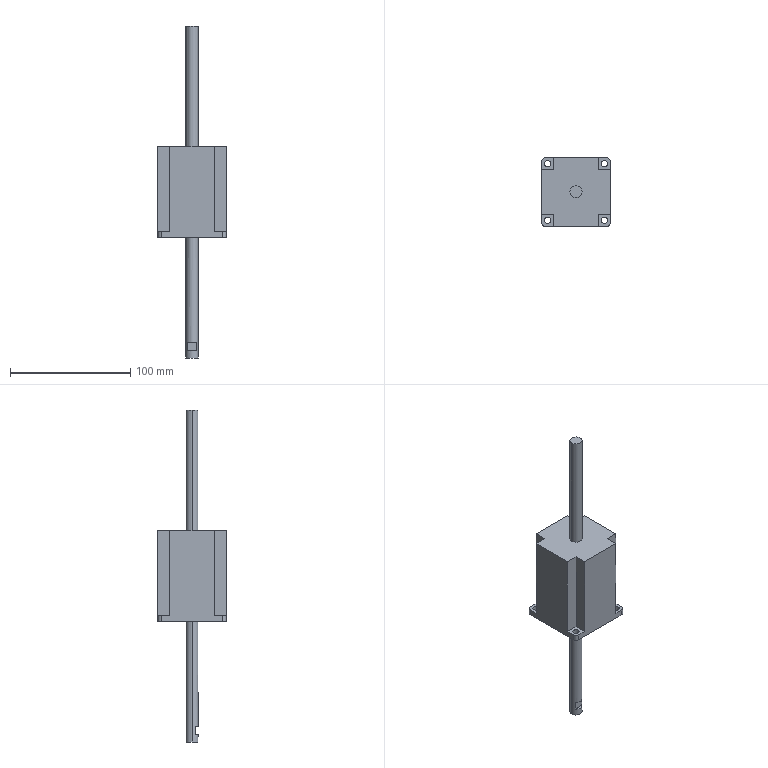Part | SolidWorks | features ICE 6, Extrusion 1, Fillet 1, MoveFace 1 | 1 solid | 39 faces | box 57 x 57 x 276 mm | volume 233690 mm3 | plane 23 | cylinder 16 | commonest cylinder face diameters 5.2 x8 6 x4 10 x4
STEP:
#1=CARTESIAN_POINT('',(5.,0.,176.));
#2=VERTEX_POINT('',#1);
#3=CARTESIAN_POINT('',(-5.,0.,176.));
#4=VERTEX_POINT('',#3);
#5=CARTESIAN_POINT('',(0.,0.,176.));
#6=DIRECTION('',(0.,0.,1.));
#7=DIRECTION('',(1.,0.,0.));
#8=AXIS2_PLACEMENT_3D('',#5,#6,#7);
#9=CIRCLE('',#8,5.);
#10=EDGE_CURVE('',#2,#4,#9,.T.);
#11=ORIENTED_EDGE('',*,*,#10,.F.);
#12=CARTESIAN_POINT('',(5.,0.,76.));
#13=VERTEX_POINT('',#12);
#14=CARTESIAN_POINT('',(5.,0.,256.));
#15=DIRECTION('',(0.,0.,-1.));
#16=VECTOR('',#15,1000.);
#17=LINE('',#14,#16);
#18=EDGE_CURVE('',#2,#13,#17,.T.);
#19=ORIENTED_EDGE('',*,*,#18,.T.);
#20=CARTESIAN_POINT('',(-5.,0.,76.));
#21=VERTEX_POINT('',#20);
#22=CARTESIAN_POINT('',(0.,0.,76.));
#23=DIRECTION('',(0.,0.,1.));
#24=DIRECTION('',(-1.,0.,0.));
#25=AXIS2_PLACEMENT_3D('',#22,#23,#24);
#26=CIRCLE('',#25,5.);
#27=EDGE_CURVE('',#13,#21,#26,.T.);
#28=ORIENTED_EDGE('',*,*,#27,.T.);
#29=CARTESIAN_POINT('',(-5.,0.,256.));
#30=DIRECTION('',(0.,0.,-1.));
#31=VECTOR('',#30,1000.);
#32=LINE('',#29,#31);
#33=EDGE_CURVE('',#4,#21,#32,.T.);
#34=ORIENTED_EDGE('',*,*,#33,.F.);
#35=EDGE_LOOP('',(#11,#19,#28,#34));
#36=FACE_OUTER_BOUND('',#35,.T.);
#37=CARTESIAN_POINT('',(0.,0.,256.));
#38=DIRECTION('',(0.,0.,-1.));
#39=DIRECTION('',(-1.,0.,0.));
#40=AXIS2_PLACEMENT_3D('',#37,#38,#39);
#41=CYLINDRICAL_SURFACE('',#40,5.);
#42=ADVANCED_FACE('',(#36),#41,.T.);
#43=CARTESIAN_POINT('',(26.15,-23.55,5.));
#44=VERTEX_POINT('',#43);
#45=CARTESIAN_POINT('',(20.95,-23.55,5.));
#46=VERTEX_POINT('',#45);
#47=CARTESIAN_POINT('',(23.55,-23.55,5.));
#48=DIRECTION('',(0.,0.,-1.));
#49=DIRECTION('',(-1.,0.,0.));
#50=AXIS2_PLACEMENT_3D('',#47,#48,#49);
#51=CIRCLE('',#50,2.6);
#52=EDGE_CURVE('',#44,#46,#51,.T.);
#53=ORIENTED_EDGE('',*,*,#52,.F.);
#54=CARTESIAN_POINT('',(26.15,-23.55,0.));
#55=VERTEX_POINT('',#54);
#56=CARTESIAN_POINT('',(26.15,-23.55,5.));
#57=DIRECTION('',(0.,0.,-1.));
#58=VECTOR('',#57,1000.);
#59=LINE('',#56,#58);
#60=EDGE_CURVE('',#44,#55,#59,.T.);
#61=ORIENTED_EDGE('',*,*,#60,.T.);
#62=CARTESIAN_POINT('',(20.95,-23.55,0.));
#63=VERTEX_POINT('',#62);
#64=CARTESIAN_POINT('',(23.55,-23.55,0.));
#65=DIRECTION('',(0.,0.,-1.));
#66=DIRECTION('',(-1.,0.,0.));
#67=AXIS2_PLACEMENT_3D('',#64,#65,#66);
#68=CIRCLE('',#67,2.6);
#69=EDGE_CURVE('',#55,#63,#68,.T.);
#70=ORIENTED_EDGE('',*,*,#69,.T.);
#71=CARTESIAN_POINT('',(20.95,-23.55,5.));
#72=DIRECTION('',(0.,0.,-1.));
#73=VECTOR('',#72,1000.);
#74=LINE('',#71,#73);
#75=EDGE_CURVE('',#46,#63,#74,.T.);
#76=ORIENTED_EDGE('',*,*,#75,.F.);
#77=EDGE_LOOP('',(#53,#61,#70,#76));
#78=FACE_OUTER_BOUND('',#77,.T.);
#79=CARTESIAN_POINT('',(23.55,-23.55,5.));
#80=DIRECTION('',(0.,0.,-1.));
#81=DIRECTION('',(-1.,0.,0.));
#82=AXIS2_PLACEMENT_3D('',#79,#80,#81);
#83=CYLINDRICAL_SURFACE('',#82,2.6);
#84=ADVANCED_FACE('',(#78),#83,.F.);
#85=CARTESIAN_POINT('',(-20.95,-23.55,5.));
#86=VERTEX_POINT('',#85);
#87=CARTESIAN_POINT('',(-26.15,-23.55,5.));
#88=VERTEX_POINT('',#87);
#89=CARTESIAN_POINT('',(-23.55,-23.55,5.));
#90=DIRECTION('',(0.,0.,-1.));
#91=DIRECTION('',(-1.,0.,0.));
#92=AXIS2_PLACEMENT_3D('',#89,#90,#91);
#93=CIRCLE('',#92,2.6);
#94=EDGE_CURVE('',#86,#88,#93,.T.);
#95=ORIENTED_EDGE('',*,*,#94,.F.);
#96=CARTESIAN_POINT('',(-20.95,-23.55,0.));
#97=VERTEX_POINT('',#96);
#98=CARTESIAN_POINT('',(-20.95,-23.55,5.));
#99=DIRECTION('',(0.,0.,-1.));
#100=VECTOR('',#99,1000.);
#101=LINE('',#98,#100);
#102=EDGE_CURVE('',#86,#97,#101,.T.);
#103=ORIENTED_EDGE('',*,*,#102,.T.);
#104=CARTESIAN_POINT('',(-26.15,-23.55,0.));
#105=VERTEX_POINT('',#104);
#106=CARTESIAN_POINT('',(-23.55,-23.55,0.));
#107=DIRECTION('',(0.,0.,-1.));
#108=DIRECTION('',(-1.,0.,0.));
#109=AXIS2_PLACEMENT_3D('',#106,#107,#108);
#110=CIRCLE('',#109,2.6);
#111=EDGE_CURVE('',#97,#105,#110,.T.);
#112=ORIENTED_EDGE('',*,*,#111,.T.);
#113=CARTESIAN_POINT('',(-26.15,-23.55,5.));
#114=DIRECTION('',(0.,0.,-1.));
#115=VECTOR('',#114,1000.);
#116=LINE('',#113,#115);
#117=EDGE_CURVE('',#88,#105,#116,.T.);
#118=ORIENTED_EDGE('',*,*,#117,.F.);
#119=EDGE_LOOP('',(#95,#103,#112,#118));
#120=FACE_OUTER_BOUND('',#119,.T.);
#121=CARTESIAN_POINT('',(-23.55,-23.55,5.));
#122=DIRECTION('',(0.,0.,-1.));
#123=DIRECTION('',(-1.,0.,0.));
#124=AXIS2_PLACEMENT_3D('',#121,#122,#123);
#125=CYLINDRICAL_SURFACE('',#124,2.6);
#126=ADVANCED_FACE('',(#120),#125,.F.);
#127=CARTESIAN_POINT('',(-20.95,23.55,5.));
#128=VERTEX_POINT('',#127);
#129=CARTESIAN_POINT('',(-26.15,23.55,5.));
#130=VERTEX_POINT('',#129);
#131=CARTESIAN_POINT('',(-23.55,23.55,5.));
#132=DIRECTION('',(0.,0.,-1.));
#133=DIRECTION('',(-1.,0.,0.));
#134=AXIS2_PLACEMENT_3D('',#131,#132,#133);
#135=CIRCLE('',#134,2.6);
#136=EDGE_CURVE('',#128,#130,#135,.T.);
#137=ORIENTED_EDGE('',*,*,#136,.F.);
#138=CARTESIAN_POINT('',(-20.95,23.55,0.));
#139=VERTEX_POINT('',#138);
#140=CARTESIAN_POINT('',(-20.95,23.55,5.));
#141=DIRECTION('',(0.,0.,-1.));
#142=VECTOR('',#141,1000.);
#143=LINE('',#140,#142);
#144=EDGE_CURVE('',#128,#139,#143,.T.);
#145=ORIENTED_EDGE('',*,*,#144,.T.);
#146=CARTESIAN_POINT('',(-26.15,23.55,0.));
#147=VERTEX_POINT('',#146);
#148=CARTESIAN_POINT('',(-23.55,23.55,0.));
#149=DIRECTION('',(0.,0.,-1.));
#150=DIRECTION('',(-1.,0.,0.));
#151=AXIS2_PLACEMENT_3D('',#148,#149,#150);
#152=CIRCLE('',#151,2.6);
#153=EDGE_CURVE('',#139,#147,#152,.T.);
#154=ORIENTED_EDGE('',*,*,#153,.T.);
#155=CARTESIAN_POINT('',(-26.15,23.55,5.));
#156=DIRECTION('',(0.,0.,-1.));
#157=VECTOR('',#156,1000.);
#158=LINE('',#155,#157);
#159=EDGE_CURVE('',#130,#147,#158,.T.);
#160=ORIENTED_EDGE('',*,*,#159,.F.);
#161=EDGE_LOOP('',(#137,#145,#154,#160));
#162=FACE_OUTER_BOUND('',#161,.T.);
#163=CARTESIAN_POINT('',(-23.55,23.55,5.));
#164=DIRECTION('',(0.,0.,-1.));
#165=DIRECTION('',(-1.,0.,0.));
#166=AXIS2_PLACEMENT_3D('',#163,#164,#165);
#167=CYLINDRICAL_SURFACE('',#166,2.6);
#168=ADVANCED_FACE('',(#162),#167,.F.);
#169=CARTESIAN_POINT('',(26.15,23.55,5.));
#170=VERTEX_POINT('',#169);
#171=CARTESIAN_POINT('',(20.95,23.55,5.));
#172=VERTEX_POINT('',#171);
#173=CARTESIAN_POINT('',(23.55,23.55,5.));
#174=DIRECTION('',(0.,0.,-1.));
#175=DIRECTION('',(-1.,0.,0.));
#176=AXIS2_PLACEMENT_3D('',#173,#174,#175);
#177=CIRCLE('',#176,2.6);
#178=EDGE_CURVE('',#170,#172,#177,.T.);
#179=ORIENTED_EDGE('',*,*,#178,.F.);
#180=CARTESIAN_POINT('',(26.15,23.55,0.));
#181=VERTEX_POINT('',#180);
#182=CARTESIAN_POINT('',(26.15,23.55,5.));
#183=DIRECTION('',(0.,0.,-1.));
#184=VECTOR('',#183,1000.);
#185=LINE('',#182,#184);
#186=EDGE_CURVE('',#170,#181,#185,.T.);
#187=ORIENTED_EDGE('',*,*,#186,.T.);
#188=CARTESIAN_POINT('',(20.95,23.55,0.));
#189=VERTEX_POINT('',#188);
#190=CARTESIAN_POINT('',(23.55,23.55,0.));
#191=DIRECTION('',(0.,0.,-1.));
#192=DIRECTION('',(-1.,0.,0.));
#193=AXIS2_PLACEMENT_3D('',#190,#191,#192);
#194=CIRCLE('',#193,2.6);
#195=EDGE_CURVE('',#181,#189,#194,.T.);
#196=ORIENTED_EDGE('',*,*,#195,.T.);
#197=CARTESIAN_POINT('',(20.95,23.55,5.));
#198=DIRECTION('',(0.,0.,-1.));
#199=VECTOR('',#198,1000.);
#200=LINE('',#197,#199);
#201=EDGE_CURVE('',#172,#189,#200,.T.);
#202=ORIENTED_EDGE('',*,*,#201,.F.);
#203=EDGE_LOOP('',(#179,#187,#196,#202));
#204=FACE_OUTER_BOUND('',#203,.T.);
#205=CARTESIAN_POINT('',(23.55,23.55,5.));
#206=DIRECTION('',(0.,0.,-1.));
#207=DIRECTION('',(-1.,0.,0.));
#208=AXIS2_PLACEMENT_3D('',#205,#206,#207);
#209=CYLINDRICAL_SURFACE('',#208,2.6);
#210=ADVANCED_FACE('',(#204),#209,.F.);
#211=CARTESIAN_POINT('',(-5.,0.,-100.));
#212=VERTEX_POINT('',#211);
#213=CARTESIAN_POINT('',(5.,0.,-100.));
#214=VERTEX_POINT('',#213);
#215=CARTESIAN_POINT('',(0.,0.,-100.));
#216=DIRECTION('',(0.,0.,-1.));
#217=DIRECTION('',(-1.,0.,0.));
#218=AXIS2_PLACEMENT_3D('',#215,#216,#217);
#219=CIRCLE('',#218,5.);
#220=EDGE_CURVE('',#212,#214,#219,.T.);
#221=ORIENTED_EDGE('',*,*,#220,.F.);
#222=CARTESIAN_POINT('',(-5.,0.,0.));
#223=VERTEX_POINT('',#222);
#224=CARTESIAN_POINT('',(-5.,0.,-20.));
#225=DIRECTION('',(0.,0.,1.));
#226=VECTOR('',#225,1000.);
#227=LINE('',#224,#226);
#228=EDGE_CURVE('',#212,#223,#227,.T.);
#229=ORIENTED_EDGE('',*,*,#228,.T.);
#230=CARTESIAN_POINT('',(5.,0.,0.));
#231=VERTEX_POINT('',#230);
#232=CARTESIAN_POINT('',(0.,0.,0.));
#233=DIRECTION('',(0.,0.,-1.));
#234=DIRECTION('',(-1.,0.,0.));
#235=AXIS2_PLACEMENT_3D('',#232,#233,#234);
#236=CIRCLE('',#235,5.);
#237=EDGE_CURVE('',#223,#231,#236,.T.);
#238=ORIENTED_EDGE('',*,*,#237,.T.);
#239=CARTESIAN_POINT('',(5.,0.,-20.));
#240=DIRECTION('',(0.,0.,1.));
#241=VECTOR('',#240,1000.);
#242=LINE('',#239,#241);
#243=EDGE_CURVE('',#214,#231,#242,.T.);
#244=ORIENTED_EDGE('',*,*,#243,.F.);
#245=EDGE_LOOP('',(#221,#229,#238,#244));
#246=FACE_OUTER_BOUND('',#245,.T.);
#247=CARTESIAN_POINT('',(0.,0.,-20.));
#248=DIRECTION('',(0.,0.,1.));
#249=DIRECTION('',(1.,0.,0.));
#250=AXIS2_PLACEMENT_3D('',#247,#248,#249);
#251=CYLINDRICAL_SURFACE('',#250,5.);
#252=ADVANCED_FACE('',(#246),#251,.T.);
#253=CARTESIAN_POINT('',(4.,-3.,-87.));
#254=VERTEX_POINT('',#253);
#255=CARTESIAN_POINT('',(-4.,-3.,-87.));
#256=VERTEX_POINT('',#255);
#257=CARTESIAN_POINT('',(7.5,-3.,-87.));
#258=DIRECTION('',(-1.,0.,0.));
#259=VECTOR('',#258,1000.);
#260=LINE('',#257,#259);
#261=EDGE_CURVE('',#254,#256,#260,.T.);
#262=ORIENTED_EDGE('',*,*,#261,.T.);
#263=CARTESIAN_POINT('',(-4.,-3.,-94.));
#264=VERTEX_POINT('',#263);
#265=CARTESIAN_POINT('',(-4.,-3.,-20.));
#266=DIRECTION('',(0.,0.,-1.));
#267=VECTOR('',#266,1000.);
#268=LINE('',#265,#267);
#269=EDGE_CURVE('',#256,#264,#268,.T.);
#270=ORIENTED_EDGE('',*,*,#269,.T.);
#271=CARTESIAN_POINT('',(4.,-3.,-94.));
#272=VERTEX_POINT('',#271);
#273=CARTESIAN_POINT('',(7.5,-3.,-94.));
#274=DIRECTION('',(-1.,0.,0.));
#275=VECTOR('',#274,1000.);
#276=LINE('',#273,#275);
#277=EDGE_CURVE('',#272,#264,#276,.T.);
#278=ORIENTED_EDGE('',*,*,#277,.F.);
#279=CARTESIAN_POINT('',(4.,-3.,-20.));
#280=DIRECTION('',(0.,0.,1.));
#281=VECTOR('',#280,1000.);
#282=LINE('',#279,#281);
#283=EDGE_CURVE('',#272,#254,#282,.T.);
#284=ORIENTED_EDGE('',*,*,#283,.T.);
#285=EDGE_LOOP('',(#262,#270,#278,#284));
#286=FACE_OUTER_BOUND('',#285,.T.);
#287=CARTESIAN_POINT('',(7.5,-3.,-7.));
#288=DIRECTION('',(0.,-1.,0.));
#289=DIRECTION('',(0.,0.,-1.));
#290=AXIS2_PLACEMENT_3D('',#287,#288,#289);
#291=PLANE('',#290);
#292=ADVANCED_FACE('',(#286),#291,.T.);
#293=ORIENTED_EDGE('',*,*,#228,.F.);
#294=CARTESIAN_POINT('',(0.,0.,-100.));
#295=DIRECTION('',(0.,0.,-1.));
#296=DIRECTION('',(-1.,0.,0.));
#297=AXIS2_PLACEMENT_3D('',#294,#295,#296);
#298=CIRCLE('',#297,5.);
#299=EDGE_CURVE('',#214,#212,#298,.T.);
#300=ORIENTED_EDGE('',*,*,#299,.F.);
#301=ORIENTED_EDGE('',*,*,#243,.T.);
#302=CARTESIAN_POINT('',(0.,0.,0.));
#303=DIRECTION('',(0.,0.,-1.));
#304=DIRECTION('',(-1.,0.,0.));
#305=AXIS2_PLACEMENT_3D('',#302,#303,#304);
#306=CIRCLE('',#305,5.);
#307=EDGE_CURVE('',#231,#223,#306,.T.);
#308=ORIENTED_EDGE('',*,*,#307,.T.);
#309=EDGE_LOOP('',(#293,#300,#301,#308));
#310=FACE_OUTER_BOUND('',#309,.T.);
#311=ORIENTED_EDGE('',*,*,#283,.F.);
#312=CARTESIAN_POINT('',(0.,0.,-94.));
#313=DIRECTION('',(0.,0.,-1.));
#314=DIRECTION('',(-1.,0.,0.));
#315=AXIS2_PLACEMENT_3D('',#312,#313,#314);
#316=CIRCLE('',#315,5.);
#317=EDGE_CURVE('',#272,#264,#316,.T.);
#318=ORIENTED_EDGE('',*,*,#317,.T.);
#319=ORIENTED_EDGE('',*,*,#269,.F.);
#320=CARTESIAN_POINT('',(0.,0.,-87.));
#321=DIRECTION('',(0.,0.,-1.));
#322=DIRECTION('',(-1.,0.,0.));
#323=AXIS2_PLACEMENT_3D('',#320,#321,#322);
#324=CIRCLE('',#323,5.);
#325=EDGE_CURVE('',#254,#256,#324,.T.);
#326=ORIENTED_EDGE('',*,*,#325,.F.);
#327=EDGE_LOOP('',(#311,#318,#319,#326));
#328=FACE_BOUND('',#327,.T.);
#329=CARTESIAN_POINT('',(0.,0.,-20.));
#330=DIRECTION('',(0.,0.,1.));
#331=DIRECTION('',(1.,0.,0.));
#332=AXIS2_PLACEMENT_3D('',#329,#330,#331);
#333=CYLINDRICAL_SURFACE('',#332,5.);
#334=ADVANCED_FACE('',(#310,#328),#333,.T.);
#335=CARTESIAN_POINT('',(28.5,-25.5,0.));
#336=VERTEX_POINT('',#335);
#337=CARTESIAN_POINT('',(28.5,25.5,0.));
#338=VERTEX_POINT('',#337);
#339=CARTESIAN_POINT('',(28.5,-28.5,0.));
#340=DIRECTION('',(0.,1.,0.));
#341=VECTOR('',#340,1000.);
#342=LINE('',#339,#341);
#343=EDGE_CURVE('',#336,#338,#342,.T.);
#344=ORIENTED_EDGE('',*,*,#343,.T.);
#345=CARTESIAN_POINT('',(28.5,25.5,5.));
#346=VERTEX_POINT('',#345);
#347=CARTESIAN_POINT('',(28.5,25.5,76.));
#348=DIRECTION('',(0.,0.,1.));
#349=VECTOR('',#348,1000.);
#350=LINE('',#347,#349);
#351=EDGE_CURVE('',#338,#346,#350,.T.);
#352=ORIENTED_EDGE('',*,*,#351,.T.);
#353=CARTESIAN_POINT('',(28.5,18.5,5.));
#354=VERTEX_POINT('',#353);
#355=CARTESIAN_POINT('',(28.5,28.5,5.));
#356=DIRECTION('',(0.,1.,0.));
#357=VECTOR('',#356,1000.);
#358=LINE('',#355,#357);
#359=EDGE_CURVE('',#354,#346,#358,.T.);
#360=ORIENTED_EDGE('',*,*,#359,.F.);
#361=CARTESIAN_POINT('',(28.5,18.5,76.));
#362=VERTEX_POINT('',#361);
#363=CARTESIAN_POINT('',(28.5,18.5,-9.142));
#364=DIRECTION('',(0.,0.,1.));
#365=VECTOR('',#364,1000.);
#366=LINE('',#363,#365);
#367=EDGE_CURVE('',#354,#362,#366,.T.);
#368=ORIENTED_EDGE('',*,*,#367,.T.);
#369=CARTESIAN_POINT('',(28.5,-18.5,76.));
#370=VERTEX_POINT('',#369);
#371=CARTESIAN_POINT('',(28.5,-28.5,76.));
#372=DIRECTION('',(0.,1.,0.));
#373=VECTOR('',#372,1000.);
#374=LINE('',#371,#373);
#375=EDGE_CURVE('',#370,#362,#374,.T.);
#376=ORIENTED_EDGE('',*,*,#375,.F.);
#377=CARTESIAN_POINT('',(28.5,-18.5,5.));
#378=VERTEX_POINT('',#377);
#379=CARTESIAN_POINT('',(28.5,-18.5,-9.142));
#380=DIRECTION('',(0.,0.,1.));
#381=VECTOR('',#380,1000.);
#382=LINE('',#379,#381);
#383=EDGE_CURVE('',#378,#370,#382,.T.);
#384=ORIENTED_EDGE('',*,*,#383,.F.);
#385=CARTESIAN_POINT('',(28.5,-25.5,5.));
#386=VERTEX_POINT('',#385);
#387=CARTESIAN_POINT('',(28.5,-28.5,5.));
#388=DIRECTION('',(0.,1.,0.));
#389=VECTOR('',#388,1000.);
#390=LINE('',#387,#389);
#391=EDGE_CURVE('',#386,#378,#390,.T.);
#392=ORIENTED_EDGE('',*,*,#391,.F.);
#393=CARTESIAN_POINT('',(28.5,-25.5,76.));
#394=DIRECTION('',(0.,0.,-1.));
#395=VECTOR('',#394,1000.);
#396=LINE('',#393,#395);
#397=EDGE_CURVE('',#386,#336,#396,.T.);
#398=ORIENTED_EDGE('',*,*,#397,.T.);
#399=EDGE_LOOP('',(#344,#352,#360,#368,#376,#384,#392,#398));
#400=FACE_OUTER_BOUND('',#399,.T.);
#401=CARTESIAN_POINT('',(28.5,-28.5,76.));
#402=DIRECTION('',(-1.,0.,0.));
#403=DIRECTION('',(0.,0.,1.));
#404=AXIS2_PLACEMENT_3D('',#401,#402,#403);
#405=PLANE('',#404);
#406=ADVANCED_FACE('',(#400),#405,.F.);
#407=CARTESIAN_POINT('',(25.5,28.5,5.));
#408=VERTEX_POINT('',#407);
#409=CARTESIAN_POINT('',(18.5,28.5,5.));
#410=VERTEX_POINT('',#409);
#411=CARTESIAN_POINT('',(28.5,28.5,5.));
#412=DIRECTION('',(-1.,0.,0.));
#413=VECTOR('',#412,1000.);
#414=LINE('',#411,#413);
#415=EDGE_CURVE('',#408,#410,#414,.T.);
#416=ORIENTED_EDGE('',*,*,#415,.F.);
#417=CARTESIAN_POINT('',(25.5,28.5,0.));
#418=VERTEX_POINT('',#417);
#419=CARTESIAN_POINT('',(25.5,28.5,76.));
#420=DIRECTION('',(0.,0.,-1.));
#421=VECTOR('',#420,1000.);
#422=LINE('',#419,#421);
#423=EDGE_CURVE('',#408,#418,#422,.T.);
#424=ORIENTED_EDGE('',*,*,#423,.T.);
#425=CARTESIAN_POINT('',(-25.5,28.5,0.));
#426=VERTEX_POINT('',#425);
#427=CARTESIAN_POINT('',(-28.5,28.5,0.));
#428=DIRECTION('',(-1.,0.,0.));
#429=VECTOR('',#428,1000.);
#430=LINE('',#427,#429);
#431=EDGE_CURVE('',#418,#426,#430,.T.);
#432=ORIENTED_EDGE('',*,*,#431,.T.);
#433=CARTESIAN_POINT('',(-25.5,28.5,5.));
#434=VERTEX_POINT('',#433);
#435=CARTESIAN_POINT('',(-25.5,28.5,76.));
#436=DIRECTION('',(0.,0.,1.));
#437=VECTOR('',#436,1000.);
#438=LINE('',#435,#437);
#439=EDGE_CURVE('',#426,#434,#438,.T.);
#440=ORIENTED_EDGE('',*,*,#439,.T.);
#441=CARTESIAN_POINT('',(-18.5,28.5,5.));
#442=VERTEX_POINT('',#441);
#443=CARTESIAN_POINT('',(-28.5,28.5,5.));
#444=DIRECTION('',(-1.,0.,0.));
#445=VECTOR('',#444,1000.);
#446=LINE('',#443,#445);
#447=EDGE_CURVE('',#442,#434,#446,.T.);
#448=ORIENTED_EDGE('',*,*,#447,.F.);
#449=CARTESIAN_POINT('',(-18.5,28.5,76.));
#450=VERTEX_POINT('',#449);
#451=CARTESIAN_POINT('',(-18.5,28.5,-9.142));
#452=DIRECTION('',(0.,0.,1.));
#453=VECTOR('',#452,1000.);
#454=LINE('',#451,#453);
#455=EDGE_CURVE('',#442,#450,#454,.T.);
#456=ORIENTED_EDGE('',*,*,#455,.T.);
#457=CARTESIAN_POINT('',(18.5,28.5,76.));
#458=VERTEX_POINT('',#457);
#459=CARTESIAN_POINT('',(-28.5,28.5,76.));
#460=DIRECTION('',(-1.,0.,0.));
#461=VECTOR('',#460,1000.);
#462=LINE('',#459,#461);
#463=EDGE_CURVE('',#458,#450,#462,.T.);
#464=ORIENTED_EDGE('',*,*,#463,.F.);
#465=CARTESIAN_POINT('',(18.5,28.5,-9.142));
#466=DIRECTION('',(0.,0.,1.));
#467=VECTOR('',#466,1000.);
#468=LINE('',#465,#467);
#469=EDGE_CURVE('',#410,#458,#468,.T.);
#470=ORIENTED_EDGE('',*,*,#469,.F.);
#471=EDGE_LOOP('',(#416,#424,#432,#440,#448,#456,#464,#470));
#472=FACE_OUTER_BOUND('',#471,.T.);
#473=CARTESIAN_POINT('',(-28.5,28.5,76.));
#474=DIRECTION('',(0.,-1.,0.));
#475=DIRECTION('',(0.,0.,-1.));
#476=AXIS2_PLACEMENT_3D('',#473,#474,#475);
#477=PLANE('',#476);
#478=ADVANCED_FACE('',(#472),#477,.F.);
#479=CARTESIAN_POINT('',(-28.5,25.5,5.));
#480=VERTEX_POINT('',#479);
#481=CARTESIAN_POINT('',(-28.5,18.5,5.));
#482=VERTEX_POINT('',#481);
#483=CARTESIAN_POINT('',(-28.5,28.5,5.));
#484=DIRECTION('',(0.,-1.,0.));
#485=VECTOR('',#484,1000.);
#486=LINE('',#483,#485);
#487=EDGE_CURVE('',#480,#482,#486,.T.);
#488=ORIENTED_EDGE('',*,*,#487,.F.);
#489=CARTESIAN_POINT('',(-28.5,25.5,0.));
#490=VERTEX_POINT('',#489);
#491=CARTESIAN_POINT('',(-28.5,25.5,76.));
#492=DIRECTION('',(0.,0.,-1.));
#493=VECTOR('',#492,1000.);
#494=LINE('',#491,#493);
#495=EDGE_CURVE('',#480,#490,#494,.T.);
#496=ORIENTED_EDGE('',*,*,#495,.T.);
#497=CARTESIAN_POINT('',(-28.5,-25.5,0.));
#498=VERTEX_POINT('',#497);
#499=CARTESIAN_POINT('',(-28.5,-28.5,0.));
#500=DIRECTION('',(0.,-1.,0.));
#501=VECTOR('',#500,1000.);
#502=LINE('',#499,#501);
#503=EDGE_CURVE('',#490,#498,#502,.T.);
#504=ORIENTED_EDGE('',*,*,#503,.T.);
#505=CARTESIAN_POINT('',(-28.5,-25.5,5.));
#506=VERTEX_POINT('',#505);
#507=CARTESIAN_POINT('',(-28.5,-25.5,76.));
#508=DIRECTION('',(0.,0.,1.));
#509=VECTOR('',#508,1000.);
#510=LINE('',#507,#509);
#511=EDGE_CURVE('',#498,#506,#510,.T.);
#512=ORIENTED_EDGE('',*,*,#511,.T.);
#513=CARTESIAN_POINT('',(-28.5,-18.5,5.));
#514=VERTEX_POINT('',#513);
#515=CARTESIAN_POINT('',(-28.5,-28.5,5.));
#516=DIRECTION('',(0.,-1.,0.));
#517=VECTOR('',#516,1000.);
#518=LINE('',#515,#517);
#519=EDGE_CURVE('',#514,#506,#518,.T.);
#520=ORIENTED_EDGE('',*,*,#519,.F.);
#521=CARTESIAN_POINT('',(-28.5,-18.5,76.));
#522=VERTEX_POINT('',#521);
#523=CARTESIAN_POINT('',(-28.5,-18.5,-9.142));
#524=DIRECTION('',(0.,0.,1.));
#525=VECTOR('',#524,1000.);
#526=LINE('',#523,#525);
#527=EDGE_CURVE('',#514,#522,#526,.T.);
#528=ORIENTED_EDGE('',*,*,#527,.T.);
#529=CARTESIAN_POINT('',(-28.5,18.5,76.));
#530=VERTEX_POINT('',#529);
#531=CARTESIAN_POINT('',(-28.5,-28.5,76.));
#532=DIRECTION('',(0.,-1.,0.));
#533=VECTOR('',#532,1000.);
#534=LINE('',#531,#533);
#535=EDGE_CURVE('',#530,#522,#534,.T.);
#536=ORIENTED_EDGE('',*,*,#535,.F.);
#537=CARTESIAN_POINT('',(-28.5,18.5,-9.142));
#538=DIRECTION('',(0.,0.,1.));
#539=VECTOR('',#538,1000.);
#540=LINE('',#537,#539);
#541=EDGE_CURVE('',#482,#530,#540,.T.);
#542=ORIENTED_EDGE('',*,*,#541,.F.);
#543=EDGE_LOOP('',(#488,#496,#504,#512,#520,#528,#536,#542));
#544=FACE_OUTER_BOUND('',#543,.T.);
#545=CARTESIAN_POINT('',(-28.5,-28.5,76.));
#546=DIRECTION('',(1.,0.,0.));
#547=DIRECTION('',(0.,0.,-1.));
#548=AXIS2_PLACEMENT_3D('',#545,#546,#547);
#549=PLANE('',#548);
#550=ADVANCED_FACE('',(#544),#549,.F.);
#551=CARTESIAN_POINT('',(-25.5,-28.5,0.));
#552=VERTEX_POINT('',#551);
#553=CARTESIAN_POINT('',(25.5,-28.5,0.));
#554=VERTEX_POINT('',#553);
#555=CARTESIAN_POINT('',(-28.5,-28.5,0.));
#556=DIRECTION('',(1.,0.,0.));
#557=VECTOR('',#556,1000.);
#558=LINE('',#555,#557);
#559=EDGE_CURVE('',#552,#554,#558,.T.);
#560=ORIENTED_EDGE('',*,*,#559,.T.);
#561=CARTESIAN_POINT('',(25.5,-28.5,5.));
#562=VERTEX_POINT('',#561);
#563=CARTESIAN_POINT('',(25.5,-28.5,76.));
#564=DIRECTION('',(0.,0.,1.));
#565=VECTOR('',#564,1000.);
#566=LINE('',#563,#565);
#567=EDGE_CURVE('',#554,#562,#566,.T.);
#568=ORIENTED_EDGE('',*,*,#567,.T.);
#569=CARTESIAN_POINT('',(18.5,-28.5,5.));
#570=VERTEX_POINT('',#569);
#571=CARTESIAN_POINT('',(28.5,-28.5,5.));
#572=DIRECTION('',(1.,0.,0.));
#573=VECTOR('',#572,1000.);
#574=LINE('',#571,#573);
#575=EDGE_CURVE('',#570,#562,#574,.T.);
#576=ORIENTED_EDGE('',*,*,#575,.F.);
#577=CARTESIAN_POINT('',(18.5,-28.5,76.));
#578=VERTEX_POINT('',#577);
#579=CARTESIAN_POINT('',(18.5,-28.5,-9.142));
#580=DIRECTION('',(0.,0.,1.));
#581=VECTOR('',#580,1000.);
#582=LINE('',#579,#581);
#583=EDGE_CURVE('',#570,#578,#582,.T.);
#584=ORIENTED_EDGE('',*,*,#583,.T.);
#585=CARTESIAN_POINT('',(-18.5,-28.5,76.));
#586=VERTEX_POINT('',#585);
#587=CARTESIAN_POINT('',(-28.5,-28.5,76.));
#588=DIRECTION('',(1.,0.,0.));
#589=VECTOR('',#588,1000.);
#590=LINE('',#587,#589);
#591=EDGE_CURVE('',#586,#578,#590,.T.);
#592=ORIENTED_EDGE('',*,*,#591,.F.);
#593=CARTESIAN_POINT('',(-18.5,-28.5,5.));
#594=VERTEX_POINT('',#593);
#595=CARTESIAN_POINT('',(-18.5,-28.5,-9.142));
#596=DIRECTION('',(0.,0.,1.));
#597=VECTOR('',#596,1000.);
#598=LINE('',#595,#597);
#599=EDGE_CURVE('',#594,#586,#598,.T.);
#600=ORIENTED_EDGE('',*,*,#599,.F.);
#601=CARTESIAN_POINT('',(-25.5,-28.5,5.));
#602=VERTEX_POINT('',#601);
#603=CARTESIAN_POINT('',(-28.5,-28.5,5.));
#604=DIRECTION('',(1.,0.,0.));
#605=VECTOR('',#604,1000.);
#606=LINE('',#603,#605);
#607=EDGE_CURVE('',#602,#594,#606,.T.);
#608=ORIENTED_EDGE('',*,*,#607,.F.);
#609=CARTESIAN_POINT('',(-25.5,-28.5,76.));
#610=DIRECTION('',(0.,0.,-1.));
#611=VECTOR('',#610,1000.);
#612=LINE('',#609,#611);
#613=EDGE_CURVE('',#602,#552,#612,.T.);
#614=ORIENTED_EDGE('',*,*,#613,.T.);
#615=EDGE_LOOP('',(#560,#568,#576,#584,#592,#600,#608,#614));
#616=FACE_OUTER_BOUND('',#615,.T.);
#617=CARTESIAN_POINT('',(-28.5,-28.5,76.));
#618=DIRECTION('',(0.,1.,0.));
#619=DIRECTION('',(0.,0.,1.));
#620=AXIS2_PLACEMENT_3D('',#617,#618,#619);
#621=PLANE('',#620);
#622=ADVANCED_FACE('',(#616),#621,.F.);
#623=CARTESIAN_POINT('',(0.,0.,76.));
#624=DIRECTION('',(0.,0.,1.));
#625=DIRECTION('',(-1.,0.,0.));
#626=AXIS2_PLACEMENT_3D('',#623,#624,#625);
#627=CIRCLE('',#626,5.);
#628=EDGE_CURVE('',#21,#13,#627,.T.);
#629=ORIENTED_EDGE('',*,*,#628,.F.);
#630=ORIENTED_EDGE('',*,*,#27,.F.);
#631=EDGE_LOOP('',(#629,#630));
#632=FACE_BOUND('',#631,.T.);
#633=CARTESIAN_POINT('',(-18.5,-18.5,76.));
#634=VERTEX_POINT('',#633);
#635=CARTESIAN_POINT('',(-28.5,-18.5,76.));
#636=DIRECTION('',(-1.,0.,0.));
#637=VECTOR('',#636,1000.);
#638=LINE('',#635,#637);
#639=EDGE_CURVE('',#634,#522,#638,.T.);
#640=ORIENTED_EDGE('',*,*,#639,.F.);
#641=CARTESIAN_POINT('',(-18.5,-28.5,76.));
#642=DIRECTION('',(0.,1.,0.));
#643=VECTOR('',#642,1000.);
#644=LINE('',#641,#643);
#645=EDGE_CURVE('',#586,#634,#644,.T.);
#646=ORIENTED_EDGE('',*,*,#645,.F.);
#647=ORIENTED_EDGE('',*,*,#591,.T.);
#648=CARTESIAN_POINT('',(18.5,-18.5,76.));
#649=VERTEX_POINT('',#648);
#650=CARTESIAN_POINT('',(18.5,-28.5,76.));
#651=DIRECTION('',(0.,-1.,0.));
#652=VECTOR('',#651,1000.);
#653=LINE('',#650,#652);
#654=EDGE_CURVE('',#649,#578,#653,.T.);
#655=ORIENTED_EDGE('',*,*,#654,.F.);
#656=CARTESIAN_POINT('',(28.5,-18.5,76.));
#657=DIRECTION('',(-1.,0.,0.));
#658=VECTOR('',#657,1000.);
#659=LINE('',#656,#658);
#660=EDGE_CURVE('',#370,#649,#659,.T.);
#661=ORIENTED_EDGE('',*,*,#660,.F.);
#662=ORIENTED_EDGE('',*,*,#375,.T.);
#663=CARTESIAN_POINT('',(18.5,18.5,76.));
#664=VERTEX_POINT('',#663);
#665=CARTESIAN_POINT('',(28.5,18.5,76.));
#666=DIRECTION('',(1.,0.,0.));
#667=VECTOR('',#666,1000.);
#668=LINE('',#665,#667);
#669=EDGE_CURVE('',#664,#362,#668,.T.);
#670=ORIENTED_EDGE('',*,*,#669,.F.);
#671=CARTESIAN_POINT('',(18.5,28.5,76.));
#672=DIRECTION('',(0.,-1.,0.));
#673=VECTOR('',#672,1000.);
#674=LINE('',#671,#673);
#675=EDGE_CURVE('',#458,#664,#674,.T.);
#676=ORIENTED_EDGE('',*,*,#675,.F.);
#677=ORIENTED_EDGE('',*,*,#463,.T.);
#678=CARTESIAN_POINT('',(-18.5,18.5,76.));
#679=VERTEX_POINT('',#678);
#680=CARTESIAN_POINT('',(-18.5,28.5,76.));
#681=DIRECTION('',(0.,1.,0.));
#682=VECTOR('',#681,1000.);
#683=LINE('',#680,#682);
#684=EDGE_CURVE('',#679,#450,#683,.T.);
#685=ORIENTED_EDGE('',*,*,#684,.F.);
#686=CARTESIAN_POINT('',(-28.5,18.5,76.));
#687=DIRECTION('',(1.,0.,0.));
#688=VECTOR('',#687,1000.);
#689=LINE('',#686,#688);
#690=EDGE_CURVE('',#530,#679,#689,.T.);
#691=ORIENTED_EDGE('',*,*,#690,.F.);
#692=ORIENTED_EDGE('',*,*,#535,.T.);
#693=EDGE_LOOP('',(#640,#646,#647,#655,#661,#662,#670,#676,#677,#685,#691,#692));
#694=FACE_OUTER_BOUND('',#693,.T.);
#695=CARTESIAN_POINT('',(0.,0.,76.));
#696=DIRECTION('',(0.,0.,-1.));
#697=DIRECTION('',(-1.,0.,0.));
#698=AXIS2_PLACEMENT_3D('',#695,#696,#697);
#699=PLANE('',#698);
#700=ADVANCED_FACE('',(#632,#694),#699,.F.);
#701=ORIENTED_EDGE('',*,*,#307,.F.);
#702=ORIENTED_EDGE('',*,*,#237,.F.);
#703=EDGE_LOOP('',(#701,#702));
#704=FACE_BOUND('',#703,.T.);
#705=CARTESIAN_POINT('',(23.55,-23.55,0.));
#706=DIRECTION('',(0.,0.,-1.));
#707=DIRECTION('',(-1.,0.,0.));
#708=AXIS2_PLACEMENT_3D('',#705,#706,#707);
#709=CIRCLE('',#708,2.6);
#710=EDGE_CURVE('',#63,#55,#709,.T.);
#711=ORIENTED_EDGE('',*,*,#710,.F.);
#712=ORIENTED_EDGE('',*,*,#69,.F.);
#713=EDGE_LOOP('',(#711,#712));
#714=FACE_BOUND('',#713,.T.);
#715=CARTESIAN_POINT('',(-23.55,-23.55,0.));
#716=DIRECTION('',(0.,0.,-1.));
#717=DIRECTION('',(-1.,0.,0.));
#718=AXIS2_PLACEMENT_3D('',#715,#716,#717);
#719=CIRCLE('',#718,2.6);
#720=EDGE_CURVE('',#105,#97,#719,.T.);
#721=ORIENTED_EDGE('',*,*,#720,.F.);
#722=ORIENTED_EDGE('',*,*,#111,.F.);
#723=EDGE_LOOP('',(#721,#722));
#724=FACE_BOUND('',#723,.T.);
#725=CARTESIAN_POINT('',(-23.55,23.55,0.));
#726=DIRECTION('',(0.,0.,-1.));
#727=DIRECTION('',(-1.,0.,0.));
#728=AXIS2_PLACEMENT_3D('',#725,#726,#727);
#729=CIRCLE('',#728,2.6);
#730=EDGE_CURVE('',#147,#139,#729,.T.);
#731=ORIENTED_EDGE('',*,*,#730,.F.);
#732=ORIENTED_EDGE('',*,*,#153,.F.);
#733=EDGE_LOOP('',(#731,#732));
#734=FACE_BOUND('',#733,.T.);
#735=CARTESIAN_POINT('',(23.55,23.55,0.));
#736=DIRECTION('',(0.,0.,-1.));
#737=DIRECTION('',(-1.,0.,0.));
#738=AXIS2_PLACEMENT_3D('',#735,#736,#737);
#739=CIRCLE('',#738,2.6);
#740=EDGE_CURVE('',#189,#181,#739,.T.);
#741=ORIENTED_EDGE('',*,*,#740,.F.);
#742=ORIENTED_EDGE('',*,*,#195,.F.);
#743=EDGE_LOOP('',(#741,#742));
#744=FACE_BOUND('',#743,.T.);
#745=ORIENTED_EDGE('',*,*,#431,.F.);
#746=CARTESIAN_POINT('',(25.5,25.5,0.));
#747=DIRECTION('',(0.,0.,-1.));
#748=DIRECTION('',(-1.,0.,0.));
#749=AXIS2_PLACEMENT_3D('',#746,#747,#748);
#750=CIRCLE('',#749,3.);
#751=EDGE_CURVE('',#418,#338,#750,.T.);
#752=ORIENTED_EDGE('',*,*,#751,.T.);
#753=ORIENTED_EDGE('',*,*,#343,.F.);
#754=CARTESIAN_POINT('',(25.5,-25.5,0.));
#755=DIRECTION('',(0.,0.,-1.));
#756=DIRECTION('',(-1.,0.,0.));
#757=AXIS2_PLACEMENT_3D('',#754,#755,#756);
#758=CIRCLE('',#757,3.);
#759=EDGE_CURVE('',#336,#554,#758,.T.);
#760=ORIENTED_EDGE('',*,*,#759,.T.);
#761=ORIENTED_EDGE('',*,*,#559,.F.);
#762=CARTESIAN_POINT('',(-25.5,-25.5,0.));
#763=DIRECTION('',(0.,0.,-1.));
#764=DIRECTION('',(-1.,0.,0.));
#765=AXIS2_PLACEMENT_3D('',#762,#763,#764);
#766=CIRCLE('',#765,3.);
#767=EDGE_CURVE('',#552,#498,#766,.T.);
#768=ORIENTED_EDGE('',*,*,#767,.T.);
#769=ORIENTED_EDGE('',*,*,#503,.F.);
#770=CARTESIAN_POINT('',(-25.5,25.5,0.));
#771=DIRECTION('',(0.,0.,-1.));
#772=DIRECTION('',(-1.,0.,0.));
#773=AXIS2_PLACEMENT_3D('',#770,#771,#772);
#774=CIRCLE('',#773,3.);
#775=EDGE_CURVE('',#490,#426,#774,.T.);
#776=ORIENTED_EDGE('',*,*,#775,.T.);
#777=EDGE_LOOP('',(#745,#752,#753,#760,#761,#768,#769,#776));
#778=FACE_OUTER_BOUND('',#777,.T.);
#779=CARTESIAN_POINT('',(0.,0.,0.));
#780=DIRECTION('',(0.,0.,-1.));
#781=DIRECTION('',(-1.,0.,0.));
#782=AXIS2_PLACEMENT_3D('',#779,#780,#781);
#783=PLANE('',#782);
#784=ADVANCED_FACE('',(#704,#714,#724,#734,#744,#778),#783,.T.);
#785=ORIENTED_EDGE('',*,*,#186,.F.);
#786=CARTESIAN_POINT('',(23.55,23.55,5.));
#787=DIRECTION('',(0.,0.,-1.));
#788=DIRECTION('',(-1.,0.,0.));
#789=AXIS2_PLACEMENT_3D('',#786,#787,#788);
#790=CIRCLE('',#789,2.6);
#791=EDGE_CURVE('',#172,#170,#790,.T.);
#792=ORIENTED_EDGE('',*,*,#791,.F.);
#793=ORIENTED_EDGE('',*,*,#201,.T.);
#794=ORIENTED_EDGE('',*,*,#740,.T.);
#795=EDGE_LOOP('',(#785,#792,#793,#794));
#796=FACE_OUTER_BOUND('',#795,.T.);
#797=CARTESIAN_POINT('',(23.55,23.55,5.));
#798=DIRECTION('',(0.,0.,-1.));
#799=DIRECTION('',(-1.,0.,0.));
#800=AXIS2_PLACEMENT_3D('',#797,#798,#799);
#801=CYLINDRICAL_SURFACE('',#800,2.6);
#802=ADVANCED_FACE('',(#796),#801,.F.);
#803=ORIENTED_EDGE('',*,*,#144,.F.);
#804=CARTESIAN_POINT('',(-23.55,23.55,5.));
#805=DIRECTION('',(0.,0.,-1.));
#806=DIRECTION('',(-1.,0.,0.));
#807=AXIS2_PLACEMENT_3D('',#804,#805,#806);
#808=CIRCLE('',#807,2.6);
#809=EDGE_CURVE('',#130,#128,#808,.T.);
#810=ORIENTED_EDGE('',*,*,#809,.F.);
#811=ORIENTED_EDGE('',*,*,#159,.T.);
#812=ORIENTED_EDGE('',*,*,#730,.T.);
#813=EDGE_LOOP('',(#803,#810,#811,#812));
#814=FACE_OUTER_BOUND('',#813,.T.);
#815=CARTESIAN_POINT('',(-23.55,23.55,5.));
#816=DIRECTION('',(0.,0.,-1.));
#817=DIRECTION('',(-1.,0.,0.));
#818=AXIS2_PLACEMENT_3D('',#815,#816,#817);
#819=CYLINDRICAL_SURFACE('',#818,2.6);
#820=ADVANCED_FACE('',(#814),#819,.F.);
#821=ORIENTED_EDGE('',*,*,#102,.F.);
#822=CARTESIAN_POINT('',(-23.55,-23.55,5.));
#823=DIRECTION('',(0.,0.,-1.));
#824=DIRECTION('',(-1.,0.,0.));
#825=AXIS2_PLACEMENT_3D('',#822,#823,#824);
#826=CIRCLE('',#825,2.6);
#827=EDGE_CURVE('',#88,#86,#826,.T.);
#828=ORIENTED_EDGE('',*,*,#827,.F.);
#829=ORIENTED_EDGE('',*,*,#117,.T.);
#830=ORIENTED_EDGE('',*,*,#720,.T.);
#831=EDGE_LOOP('',(#821,#828,#829,#830));
#832=FACE_OUTER_BOUND('',#831,.T.);
#833=CARTESIAN_POINT('',(-23.55,-23.55,5.));
#834=DIRECTION('',(0.,0.,-1.));
#835=DIRECTION('',(-1.,0.,0.));
#836=AXIS2_PLACEMENT_3D('',#833,#834,#835);
#837=CYLINDRICAL_SURFACE('',#836,2.6);
#838=ADVANCED_FACE('',(#832),#837,.F.);
#839=ORIENTED_EDGE('',*,*,#60,.F.);
#840=CARTESIAN_POINT('',(23.55,-23.55,5.));
#841=DIRECTION('',(0.,0.,-1.));
#842=DIRECTION('',(-1.,0.,0.));
#843=AXIS2_PLACEMENT_3D('',#840,#841,#842);
#844=CIRCLE('',#843,2.6);
#845=EDGE_CURVE('',#46,#44,#844,.T.);
#846=ORIENTED_EDGE('',*,*,#845,.F.);
#847=ORIENTED_EDGE('',*,*,#75,.T.);
#848=ORIENTED_EDGE('',*,*,#710,.T.);
#849=EDGE_LOOP('',(#839,#846,#847,#848));
#850=FACE_OUTER_BOUND('',#849,.T.);
#851=CARTESIAN_POINT('',(23.55,-23.55,5.));
#852=DIRECTION('',(0.,0.,-1.));
#853=DIRECTION('',(-1.,0.,0.));
#854=AXIS2_PLACEMENT_3D('',#851,#852,#853);
#855=CYLINDRICAL_SURFACE('',#854,2.6);
#856=ADVANCED_FACE('',(#850),#855,.F.);
#857=ORIENTED_EDGE('',*,*,#299,.T.);
#858=ORIENTED_EDGE('',*,*,#220,.T.);
#859=EDGE_LOOP('',(#857,#858));
#860=FACE_OUTER_BOUND('',#859,.T.);
#861=CARTESIAN_POINT('',(0.,0.,-100.));
#862=DIRECTION('',(0.,0.,-1.));
#863=DIRECTION('',(-1.,0.,0.));
#864=AXIS2_PLACEMENT_3D('',#861,#862,#863);
#865=PLANE('',#864);
#866=ADVANCED_FACE('',(#860),#865,.T.);
#867=ORIENTED_EDGE('',*,*,#18,.F.);
#868=CARTESIAN_POINT('',(0.,0.,176.));
#869=DIRECTION('',(0.,0.,1.));
#870=DIRECTION('',(1.,0.,0.));
#871=AXIS2_PLACEMENT_3D('',#868,#869,#870);
#872=CIRCLE('',#871,5.);
#873=EDGE_CURVE('',#4,#2,#872,.T.);
#874=ORIENTED_EDGE('',*,*,#873,.F.);
#875=ORIENTED_EDGE('',*,*,#33,.T.);
#876=ORIENTED_EDGE('',*,*,#628,.T.);
#877=EDGE_LOOP('',(#867,#874,#875,#876));
#878=FACE_OUTER_BOUND('',#877,.T.);
#879=CARTESIAN_POINT('',(0.,0.,256.));
#880=DIRECTION('',(0.,0.,-1.));
#881=DIRECTION('',(-1.,0.,0.));
#882=AXIS2_PLACEMENT_3D('',#879,#880,#881);
#883=CYLINDRICAL_SURFACE('',#882,5.);
#884=ADVANCED_FACE('',(#878),#883,.T.);
#885=ORIENTED_EDGE('',*,*,#873,.T.);
#886=ORIENTED_EDGE('',*,*,#10,.T.);
#887=EDGE_LOOP('',(#885,#886));
#888=FACE_OUTER_BOUND('',#887,.T.);
#889=CARTESIAN_POINT('',(0.,0.,176.));
#890=DIRECTION('',(0.,0.,1.));
#891=DIRECTION('',(1.,0.,0.));
#892=AXIS2_PLACEMENT_3D('',#889,#890,#891);
#893=PLANE('',#892);
#894=ADVANCED_FACE('',(#888),#893,.T.);
#895=ORIENTED_EDGE('',*,*,#325,.T.);
#896=ORIENTED_EDGE('',*,*,#261,.F.);
#897=EDGE_LOOP('',(#895,#896));
#898=FACE_OUTER_BOUND('',#897,.T.);
#899=CARTESIAN_POINT('',(0.,0.,-87.));
#900=DIRECTION('',(0.,0.,-1.));
#901=DIRECTION('',(-1.,0.,0.));
#902=AXIS2_PLACEMENT_3D('',#899,#900,#901);
#903=PLANE('',#902);
#904=ADVANCED_FACE('',(#898),#903,.T.);
#905=ORIENTED_EDGE('',*,*,#277,.T.);
#906=ORIENTED_EDGE('',*,*,#317,.F.);
#907=EDGE_LOOP('',(#905,#906));
#908=FACE_OUTER_BOUND('',#907,.T.);
#909=CARTESIAN_POINT('',(0.,0.,-94.));
#910=DIRECTION('',(0.,0.,-1.));
#911=DIRECTION('',(-1.,0.,0.));
#912=AXIS2_PLACEMENT_3D('',#909,#910,#911);
#913=PLANE('',#912);
#914=ADVANCED_FACE('',(#908),#913,.F.);
#915=ORIENTED_EDGE('',*,*,#809,.T.);
#916=ORIENTED_EDGE('',*,*,#136,.T.);
#917=EDGE_LOOP('',(#915,#916));
#918=FACE_BOUND('',#917,.T.);
#919=ORIENTED_EDGE('',*,*,#447,.T.);
#920=CARTESIAN_POINT('',(-25.5,25.5,5.));
#921=DIRECTION('',(0.,0.,1.));
#922=DIRECTION('',(-1.,0.,0.));
#923=AXIS2_PLACEMENT_3D('',#920,#921,#922);
#924=CIRCLE('',#923,3.);
#925=EDGE_CURVE('',#434,#480,#924,.T.);
#926=ORIENTED_EDGE('',*,*,#925,.T.);
#927=ORIENTED_EDGE('',*,*,#487,.T.);
#928=CARTESIAN_POINT('',(-18.5,18.5,5.));
#929=VERTEX_POINT('',#928);
#930=CARTESIAN_POINT('',(-28.5,18.5,5.));
#931=DIRECTION('',(1.,0.,0.));
#932=VECTOR('',#931,1000.);
#933=LINE('',#930,#932);
#934=EDGE_CURVE('',#482,#929,#933,.T.);
#935=ORIENTED_EDGE('',*,*,#934,.T.);
#936=CARTESIAN_POINT('',(-18.5,28.5,5.));
#937=DIRECTION('',(0.,1.,0.));
#938=VECTOR('',#937,1000.);
#939=LINE('',#936,#938);
#940=EDGE_CURVE('',#929,#442,#939,.T.);
#941=ORIENTED_EDGE('',*,*,#940,.T.);
#942=EDGE_LOOP('',(#919,#926,#927,#935,#941));
#943=FACE_OUTER_BOUND('',#942,.T.);
#944=CARTESIAN_POINT('',(-23.55,23.55,5.));
#945=DIRECTION('',(0.,0.,-1.));
#946=DIRECTION('',(-1.,0.,0.));
#947=AXIS2_PLACEMENT_3D('',#944,#945,#946);
#948=PLANE('',#947);
#949=ADVANCED_FACE('',(#918,#943),#948,.F.);
#950=ORIENTED_EDGE('',*,*,#541,.T.);
#951=ORIENTED_EDGE('',*,*,#690,.T.);
#952=CARTESIAN_POINT('',(-18.5,18.5,-9.142));
#953=DIRECTION('',(0.,0.,1.));
#954=VECTOR('',#953,1000.);
#955=LINE('',#952,#954);
#956=EDGE_CURVE('',#929,#679,#955,.T.);
#957=ORIENTED_EDGE('',*,*,#956,.F.);
#958=ORIENTED_EDGE('',*,*,#934,.F.);
#959=EDGE_LOOP('',(#950,#951,#957,#958));
#960=FACE_OUTER_BOUND('',#959,.T.);
#961=CARTESIAN_POINT('',(-28.5,18.5,-9.142));
#962=DIRECTION('',(0.,-1.,0.));
#963=DIRECTION('',(0.,0.,-1.));
#964=AXIS2_PLACEMENT_3D('',#961,#962,#963);
#965=PLANE('',#964);
#966=ADVANCED_FACE('',(#960),#965,.F.);
#967=ORIENTED_EDGE('',*,*,#956,.T.);
#968=ORIENTED_EDGE('',*,*,#684,.T.);
#969=ORIENTED_EDGE('',*,*,#455,.F.);
#970=ORIENTED_EDGE('',*,*,#940,.F.);
#971=EDGE_LOOP('',(#967,#968,#969,#970));
#972=FACE_OUTER_BOUND('',#971,.T.);
#973=CARTESIAN_POINT('',(-18.5,28.5,-9.142));
#974=DIRECTION('',(1.,0.,0.));
#975=DIRECTION('',(0.,0.,-1.));
#976=AXIS2_PLACEMENT_3D('',#973,#974,#975);
#977=PLANE('',#976);
#978=ADVANCED_FACE('',(#972),#977,.F.);
#979=ORIENTED_EDGE('',*,*,#791,.T.);
#980=ORIENTED_EDGE('',*,*,#178,.T.);
#981=EDGE_LOOP('',(#979,#980));
#982=FACE_BOUND('',#981,.T.);
#983=ORIENTED_EDGE('',*,*,#359,.T.);
#984=CARTESIAN_POINT('',(25.5,25.5,5.));
#985=DIRECTION('',(0.,0.,1.));
#986=DIRECTION('',(-1.,0.,0.));
#987=AXIS2_PLACEMENT_3D('',#984,#985,#986);
#988=CIRCLE('',#987,3.);
#989=EDGE_CURVE('',#346,#408,#988,.T.);
#990=ORIENTED_EDGE('',*,*,#989,.T.);
#991=ORIENTED_EDGE('',*,*,#415,.T.);
#992=CARTESIAN_POINT('',(18.5,18.5,5.));
#993=VERTEX_POINT('',#992);
#994=CARTESIAN_POINT('',(18.5,28.5,5.));
#995=DIRECTION('',(0.,-1.,0.));
#996=VECTOR('',#995,1000.);
#997=LINE('',#994,#996);
#998=EDGE_CURVE('',#410,#993,#997,.T.);
#999=ORIENTED_EDGE('',*,*,#998,.T.);
#1000=CARTESIAN_POINT('',(28.5,18.5,5.));
#1001=DIRECTION('',(1.,0.,0.));
#1002=VECTOR('',#1001,1000.);
#1003=LINE('',#1000,#1002);
#1004=EDGE_CURVE('',#993,#354,#1003,.T.);
#1005=ORIENTED_EDGE('',*,*,#1004,.T.);
#1006=EDGE_LOOP('',(#983,#990,#991,#999,#1005));
#1007=FACE_OUTER_BOUND('',#1006,.T.);
#1008=CARTESIAN_POINT('',(-23.55,23.55,5.));
#1009=DIRECTION('',(0.,0.,-1.));
#1010=DIRECTION('',(-1.,0.,0.));
#1011=AXIS2_PLACEMENT_3D('',#1008,#1009,#1010);
#1012=PLANE('',#1011);
#1013=ADVANCED_FACE('',(#982,#1007),#1012,.F.);
#1014=ORIENTED_EDGE('',*,*,#469,.T.);
#1015=ORIENTED_EDGE('',*,*,#675,.T.);
#1016=CARTESIAN_POINT('',(18.5,18.5,-9.142));
#1017=DIRECTION('',(0.,0.,1.));
#1018=VECTOR('',#1017,1000.);
#1019=LINE('',#1016,#1018);
#1020=EDGE_CURVE('',#993,#664,#1019,.T.);
#1021=ORIENTED_EDGE('',*,*,#1020,.F.);
#1022=ORIENTED_EDGE('',*,*,#998,.F.);
#1023=EDGE_LOOP('',(#1014,#1015,#1021,#1022));
#1024=FACE_OUTER_BOUND('',#1023,.T.);
#1025=CARTESIAN_POINT('',(18.5,28.5,-9.142));
#1026=DIRECTION('',(-1.,0.,0.));
#1027=DIRECTION('',(0.,-1.,0.));
#1028=AXIS2_PLACEMENT_3D('',#1025,#1026,#1027);
#1029=PLANE('',#1028);
#1030=ADVANCED_FACE('',(#1024),#1029,.F.);
#1031=ORIENTED_EDGE('',*,*,#1020,.T.);
#1032=ORIENTED_EDGE('',*,*,#669,.T.);
#1033=ORIENTED_EDGE('',*,*,#367,.F.);
#1034=ORIENTED_EDGE('',*,*,#1004,.F.);
#1035=EDGE_LOOP('',(#1031,#1032,#1033,#1034));
#1036=FACE_OUTER_BOUND('',#1035,.T.);
#1037=CARTESIAN_POINT('',(28.5,18.5,-9.142));
#1038=DIRECTION('',(0.,-1.,0.));
#1039=DIRECTION('',(1.,0.,0.));
#1040=AXIS2_PLACEMENT_3D('',#1037,#1038,#1039);
#1041=PLANE('',#1040);
#1042=ADVANCED_FACE('',(#1036),#1041,.F.);
#1043=ORIENTED_EDGE('',*,*,#845,.T.);
#1044=ORIENTED_EDGE('',*,*,#52,.T.);
#1045=EDGE_LOOP('',(#1043,#1044));
#1046=FACE_BOUND('',#1045,.T.);
#1047=ORIENTED_EDGE('',*,*,#575,.T.);
#1048=CARTESIAN_POINT('',(25.5,-25.5,5.));
#1049=DIRECTION('',(0.,0.,1.));
#1050=DIRECTION('',(-1.,0.,0.));
#1051=AXIS2_PLACEMENT_3D('',#1048,#1049,#1050);
#1052=CIRCLE('',#1051,3.);
#1053=EDGE_CURVE('',#562,#386,#1052,.T.);
#1054=ORIENTED_EDGE('',*,*,#1053,.T.);
#1055=ORIENTED_EDGE('',*,*,#391,.T.);
#1056=CARTESIAN_POINT('',(18.5,-18.5,5.));
#1057=VERTEX_POINT('',#1056);
#1058=CARTESIAN_POINT('',(28.5,-18.5,5.));
#1059=DIRECTION('',(-1.,0.,0.));
#1060=VECTOR('',#1059,1000.);
#1061=LINE('',#1058,#1060);
#1062=EDGE_CURVE('',#378,#1057,#1061,.T.);
#1063=ORIENTED_EDGE('',*,*,#1062,.T.);
#1064=CARTESIAN_POINT('',(18.5,-28.5,5.));
#1065=DIRECTION('',(0.,-1.,0.));
#1066=VECTOR('',#1065,1000.);
#1067=LINE('',#1064,#1066);
#1068=EDGE_CURVE('',#1057,#570,#1067,.T.);
#1069=ORIENTED_EDGE('',*,*,#1068,.T.);
#1070=EDGE_LOOP('',(#1047,#1054,#1055,#1063,#1069));
#1071=FACE_OUTER_BOUND('',#1070,.T.);
#1072=CARTESIAN_POINT('',(-23.55,23.55,5.));
#1073=DIRECTION('',(0.,0.,-1.));
#1074=DIRECTION('',(-1.,0.,0.));
#1075=AXIS2_PLACEMENT_3D('',#1072,#1073,#1074);
#1076=PLANE('',#1075);
#1077=ADVANCED_FACE('',(#1046,#1071),#1076,.F.);
#1078=ORIENTED_EDGE('',*,*,#383,.T.);
#1079=ORIENTED_EDGE('',*,*,#660,.T.);
#1080=CARTESIAN_POINT('',(18.5,-18.5,-9.142));
#1081=DIRECTION('',(0.,0.,1.));
#1082=VECTOR('',#1081,1000.);
#1083=LINE('',#1080,#1082);
#1084=EDGE_CURVE('',#1057,#649,#1083,.T.);
#1085=ORIENTED_EDGE('',*,*,#1084,.F.);
#1086=ORIENTED_EDGE('',*,*,#1062,.F.);
#1087=EDGE_LOOP('',(#1078,#1079,#1085,#1086));
#1088=FACE_OUTER_BOUND('',#1087,.T.);
#1089=CARTESIAN_POINT('',(28.5,-18.5,-9.142));
#1090=DIRECTION('',(0.,1.,0.));
#1091=DIRECTION('',(0.,0.,1.));
#1092=AXIS2_PLACEMENT_3D('',#1089,#1090,#1091);
#1093=PLANE('',#1092);
#1094=ADVANCED_FACE('',(#1088),#1093,.F.);
#1095=ORIENTED_EDGE('',*,*,#1084,.T.);
#1096=ORIENTED_EDGE('',*,*,#654,.T.);
#1097=ORIENTED_EDGE('',*,*,#583,.F.);
#1098=ORIENTED_EDGE('',*,*,#1068,.F.);
#1099=EDGE_LOOP('',(#1095,#1096,#1097,#1098));
#1100=FACE_OUTER_BOUND('',#1099,.T.);
#1101=CARTESIAN_POINT('',(18.5,-28.5,-9.142));
#1102=DIRECTION('',(-1.,0.,0.));
#1103=DIRECTION('',(0.,0.,1.));
#1104=AXIS2_PLACEMENT_3D('',#1101,#1102,#1103);
#1105=PLANE('',#1104);
#1106=ADVANCED_FACE('',(#1100),#1105,.F.);
#1107=ORIENTED_EDGE('',*,*,#827,.T.);
#1108=ORIENTED_EDGE('',*,*,#94,.T.);
#1109=EDGE_LOOP('',(#1107,#1108));
#1110=FACE_BOUND('',#1109,.T.);
#1111=ORIENTED_EDGE('',*,*,#519,.T.);
#1112=CARTESIAN_POINT('',(-25.5,-25.5,5.));
#1113=DIRECTION('',(0.,0.,1.));
#1114=DIRECTION('',(-1.,0.,0.));
#1115=AXIS2_PLACEMENT_3D('',#1112,#1113,#1114);
#1116=CIRCLE('',#1115,3.);
#1117=EDGE_CURVE('',#506,#602,#1116,.T.);
#1118=ORIENTED_EDGE('',*,*,#1117,.T.);
#1119=ORIENTED_EDGE('',*,*,#607,.T.);
#1120=CARTESIAN_POINT('',(-18.5,-18.5,5.));
#1121=VERTEX_POINT('',#1120);
#1122=CARTESIAN_POINT('',(-18.5,-28.5,5.));
#1123=DIRECTION('',(0.,1.,0.));
#1124=VECTOR('',#1123,1000.);
#1125=LINE('',#1122,#1124);
#1126=EDGE_CURVE('',#594,#1121,#1125,.T.);
#1127=ORIENTED_EDGE('',*,*,#1126,.T.);
#1128=CARTESIAN_POINT('',(-28.5,-18.5,5.));
#1129=DIRECTION('',(-1.,0.,0.));
#1130=VECTOR('',#1129,1000.);
#1131=LINE('',#1128,#1130);
#1132=EDGE_CURVE('',#1121,#514,#1131,.T.);
#1133=ORIENTED_EDGE('',*,*,#1132,.T.);
#1134=EDGE_LOOP('',(#1111,#1118,#1119,#1127,#1133));
#1135=FACE_OUTER_BOUND('',#1134,.T.);
#1136=CARTESIAN_POINT('',(-23.55,23.55,5.));
#1137=DIRECTION('',(0.,0.,-1.));
#1138=DIRECTION('',(-1.,0.,0.));
#1139=AXIS2_PLACEMENT_3D('',#1136,#1137,#1138);
#1140=PLANE('',#1139);
#1141=ADVANCED_FACE('',(#1110,#1135),#1140,.F.);
#1142=ORIENTED_EDGE('',*,*,#599,.T.);
#1143=ORIENTED_EDGE('',*,*,#645,.T.);
#1144=CARTESIAN_POINT('',(-18.5,-18.5,-9.142));
#1145=DIRECTION('',(0.,0.,1.));
#1146=VECTOR('',#1145,1000.);
#1147=LINE('',#1144,#1146);
#1148=EDGE_CURVE('',#1121,#634,#1147,.T.);
#1149=ORIENTED_EDGE('',*,*,#1148,.F.);
#1150=ORIENTED_EDGE('',*,*,#1126,.F.);
#1151=EDGE_LOOP('',(#1142,#1143,#1149,#1150));
#1152=FACE_OUTER_BOUND('',#1151,.T.);
#1153=CARTESIAN_POINT('',(-18.5,-28.5,-9.142));
#1154=DIRECTION('',(1.,0.,0.));
#1155=DIRECTION('',(0.,1.,0.));
#1156=AXIS2_PLACEMENT_3D('',#1153,#1154,#1155);
#1157=PLANE('',#1156);
#1158=ADVANCED_FACE('',(#1152),#1157,.F.);
#1159=ORIENTED_EDGE('',*,*,#1148,.T.);
#1160=ORIENTED_EDGE('',*,*,#639,.T.);
#1161=ORIENTED_EDGE('',*,*,#527,.F.);
#1162=ORIENTED_EDGE('',*,*,#1132,.F.);
#1163=EDGE_LOOP('',(#1159,#1160,#1161,#1162));
#1164=FACE_OUTER_BOUND('',#1163,.T.);
#1165=CARTESIAN_POINT('',(-28.5,-18.5,-9.142));
#1166=DIRECTION('',(0.,1.,0.));
#1167=DIRECTION('',(-1.,0.,0.));
#1168=AXIS2_PLACEMENT_3D('',#1165,#1166,#1167);
#1169=PLANE('',#1168);
#1170=ADVANCED_FACE('',(#1164),#1169,.F.);
#1171=ORIENTED_EDGE('',*,*,#989,.F.);
#1172=ORIENTED_EDGE('',*,*,#351,.F.);
#1173=ORIENTED_EDGE('',*,*,#751,.F.);
#1174=ORIENTED_EDGE('',*,*,#423,.F.);
#1175=EDGE_LOOP('',(#1171,#1172,#1173,#1174));
#1176=FACE_OUTER_BOUND('',#1175,.T.);
#1177=CARTESIAN_POINT('',(25.5,25.5,76.));
#1178=DIRECTION('',(0.,0.,-1.));
#1179=DIRECTION('',(-1.,0.,0.));
#1180=AXIS2_PLACEMENT_3D('',#1177,#1178,#1179);
#1181=CYLINDRICAL_SURFACE('',#1180,3.);
#1182=ADVANCED_FACE('',(#1176),#1181,.T.);
#1183=ORIENTED_EDGE('',*,*,#925,.F.);
#1184=ORIENTED_EDGE('',*,*,#439,.F.);
#1185=ORIENTED_EDGE('',*,*,#775,.F.);
#1186=ORIENTED_EDGE('',*,*,#495,.F.);
#1187=EDGE_LOOP('',(#1183,#1184,#1185,#1186));
#1188=FACE_OUTER_BOUND('',#1187,.T.);
#1189=CARTESIAN_POINT('',(-25.5,25.5,76.));
#1190=DIRECTION('',(0.,0.,-1.));
#1191=DIRECTION('',(-1.,0.,0.));
#1192=AXIS2_PLACEMENT_3D('',#1189,#1190,#1191);
#1193=CYLINDRICAL_SURFACE('',#1192,3.);
#1194=ADVANCED_FACE('',(#1188),#1193,.T.);
#1195=ORIENTED_EDGE('',*,*,#1053,.F.);
#1196=ORIENTED_EDGE('',*,*,#567,.F.);
#1197=ORIENTED_EDGE('',*,*,#759,.F.);
#1198=ORIENTED_EDGE('',*,*,#397,.F.);
#1199=EDGE_LOOP('',(#1195,#1196,#1197,#1198));
#1200=FACE_OUTER_BOUND('',#1199,.T.);
#1201=CARTESIAN_POINT('',(25.5,-25.5,76.));
#1202=DIRECTION('',(0.,0.,-1.));
#1203=DIRECTION('',(-1.,0.,0.));
#1204=AXIS2_PLACEMENT_3D('',#1201,#1202,#1203);
#1205=CYLINDRICAL_SURFACE('',#1204,3.);
#1206=ADVANCED_FACE('',(#1200),#1205,.T.);
#1207=ORIENTED_EDGE('',*,*,#1117,.F.);
#1208=ORIENTED_EDGE('',*,*,#511,.F.);
#1209=ORIENTED_EDGE('',*,*,#767,.F.);
#1210=ORIENTED_EDGE('',*,*,#613,.F.);
#1211=EDGE_LOOP('',(#1207,#1208,#1209,#1210));
#1212=FACE_OUTER_BOUND('',#1211,.T.);
#1213=CARTESIAN_POINT('',(-25.5,-25.5,76.));
#1214=DIRECTION('',(0.,0.,-1.));
#1215=DIRECTION('',(-1.,0.,0.));
#1216=AXIS2_PLACEMENT_3D('',#1213,#1214,#1215);
#1217=CYLINDRICAL_SURFACE('',#1216,3.);
#1218=ADVANCED_FACE('',(#1212),#1217,.T.);
#1219=CLOSED_SHELL('',(#42,#84,#126,#168,#210,#252,#292,#334,#406,#478,#550,#622,#700,#784,#802,#820,#838,#856,#866,#884,#894,#904,#914,#949,#966,#978,#1013,#1030,#1042,#1077,#1094,#1106,#1141,#1158,#1170,#1182,#1194,#1206,#1218));
#1220=MANIFOLD_SOLID_BREP('',#1219);
#1221=CARTESIAN_POINT('',(0.,0.,0.));
#1222=DIRECTION('',(0.,0.,1.));
#1223=DIRECTION('',(1.,0.,0.));
#1224=AXIS2_PLACEMENT_3D('',#1221,#1222,#1223);
#1225=(LENGTH_UNIT()NAMED_UNIT(*)SI_UNIT(.MILLI.,.METRE.));
#1226=UNCERTAINTY_MEASURE_WITH_UNIT(LENGTH_MEASURE(0.00001),#1225,'','');
#1227=(NAMED_UNIT(*)PLANE_ANGLE_UNIT()SI_UNIT($,.RADIAN.));
#1228=(NAMED_UNIT(*)SI_UNIT($,.STERADIAN.)SOLID_ANGLE_UNIT());
#1229=(GEOMETRIC_REPRESENTATION_CONTEXT(3)GLOBAL_UNCERTAINTY_ASSIGNED_CONTEXT((#1226))GLOBAL_UNIT_ASSIGNED_CONTEXT((#1225,#1227,#1228))REPRESENTATION_CONTEXT('',''));
#1230=ADVANCED_BREP_SHAPE_REPRESENTATION('',(#1220,#1224),#1229);